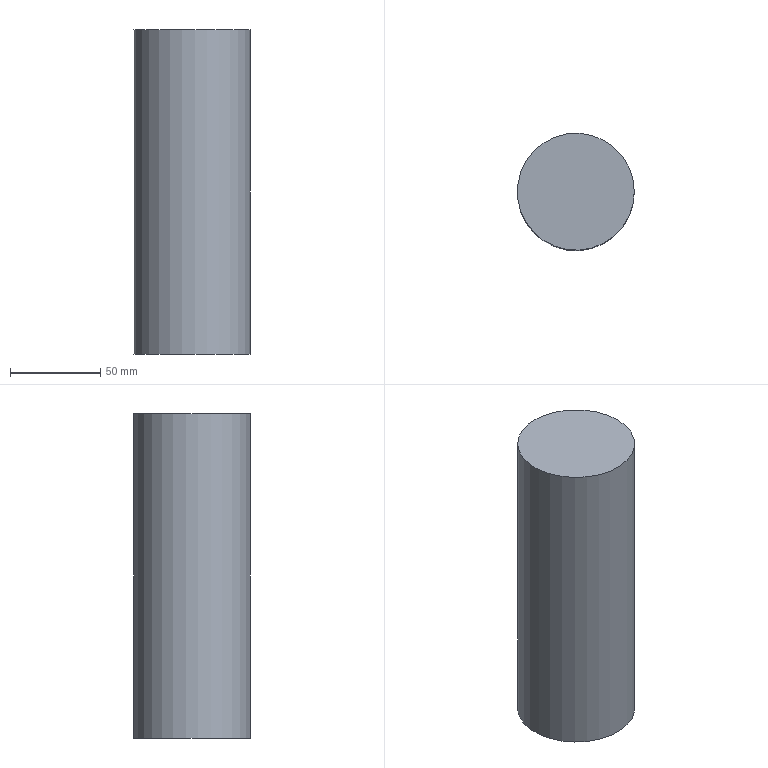Part | NX | features solid 2 | 1 solid | 3 faces | box 65 x 65 x 180 mm | volume 597295 mm3 | plane 2 | cylinder 1 | commonest cylinder face diameters 65 x1
STEP:
#1=CARTESIAN_POINT('',(2162.5,265.,-196.));
#2=VERTEX_POINT('',#1);
#3=CARTESIAN_POINT('',(2130.,265.,-196.));
#4=DIRECTION('',(0.,0.,1.));
#5=DIRECTION('',(1.,0.,0.));
#6=AXIS2_PLACEMENT_3D('',#3,#4,#5);
#7=CIRCLE('',#6,32.5);
#8=EDGE_CURVE('',#2,#2,#7,.T.);
#9=ORIENTED_EDGE('',*,*,#8,.T.);
#10=EDGE_LOOP('',(#9));
#11=FACE_BOUND('',#10,.T.);
#12=CARTESIAN_POINT('',(2162.5,265.,-16.));
#13=VERTEX_POINT('',#12);
#14=CARTESIAN_POINT('',(2130.,265.,-16.));
#15=DIRECTION('',(0.,0.,1.));
#16=DIRECTION('',(1.,0.,0.));
#17=AXIS2_PLACEMENT_3D('',#14,#15,#16);
#18=CIRCLE('',#17,32.5);
#19=EDGE_CURVE('',#13,#13,#18,.T.);
#20=ORIENTED_EDGE('',*,*,#19,.F.);
#21=EDGE_LOOP('',(#20));
#22=FACE_BOUND('',#21,.T.);
#23=CARTESIAN_POINT('',(2130.,265.,-3.75));
#24=DIRECTION('',(0.,0.,1.));
#25=DIRECTION('',(0.,1.,0.));
#26=AXIS2_PLACEMENT_3D('',#23,#24,#25);
#27=CYLINDRICAL_SURFACE('',#26,32.5);
#28=ADVANCED_FACE('',(#11,#22),#27,.T.);
#29=ORIENTED_EDGE('',*,*,#8,.F.);
#30=EDGE_LOOP('',(#29));
#31=FACE_BOUND('',#30,.T.);
#32=CARTESIAN_POINT('',(2145.5,265.,-196.));
#33=DIRECTION('',(0.,0.,-1.));
#34=DIRECTION('',(0.,-1.,0.));
#35=AXIS2_PLACEMENT_3D('',#32,#33,#34);
#36=PLANE('',#35);
#37=ADVANCED_FACE('',(#31),#36,.T.);
#38=ORIENTED_EDGE('',*,*,#19,.T.);
#39=EDGE_LOOP('',(#38));
#40=FACE_BOUND('',#39,.T.);
#41=CARTESIAN_POINT('',(2145.5,265.,-16.));
#42=DIRECTION('',(0.,0.,-1.));
#43=DIRECTION('',(0.,-1.,0.));
#44=AXIS2_PLACEMENT_3D('',#41,#42,#43);
#45=PLANE('',#44);
#46=ADVANCED_FACE('',(#40),#45,.F.);
#47=CLOSED_SHELL('',(#28,#37,#46));
#48=MANIFOLD_SOLID_BREP('',#47);
#49=(LENGTH_UNIT()NAMED_UNIT(*)SI_UNIT(.MILLI.,.METRE.));
#50=UNCERTAINTY_MEASURE_WITH_UNIT(LENGTH_MEASURE(0.00001),#49,'','');
#51=(NAMED_UNIT(*)PLANE_ANGLE_UNIT()SI_UNIT($,.RADIAN.));
#52=(NAMED_UNIT(*)SI_UNIT($,.STERADIAN.)SOLID_ANGLE_UNIT());
#53=(GEOMETRIC_REPRESENTATION_CONTEXT(3)GLOBAL_UNCERTAINTY_ASSIGNED_CONTEXT((#50))GLOBAL_UNIT_ASSIGNED_CONTEXT((#49,#51,#52))REPRESENTATION_CONTEXT('',''));
#54=ADVANCED_BREP_SHAPE_REPRESENTATION('',(#48),#53);